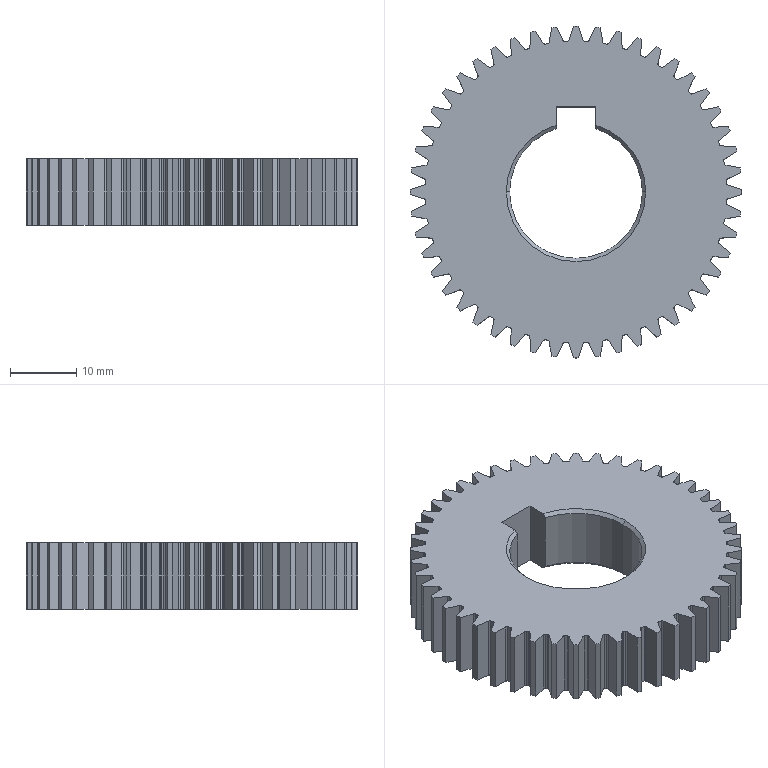Part | SolidWorks | features BaseBody 1, RefAxis 1 | 1 solid | 323 faces | box 50 x 50 x 10 mm | volume 14543 mm3 | cylinder 216 | plane 101 | cone 6 | commonest cylinder face diameters 0.5 x116 50 x49 45.5 x48 20 x3